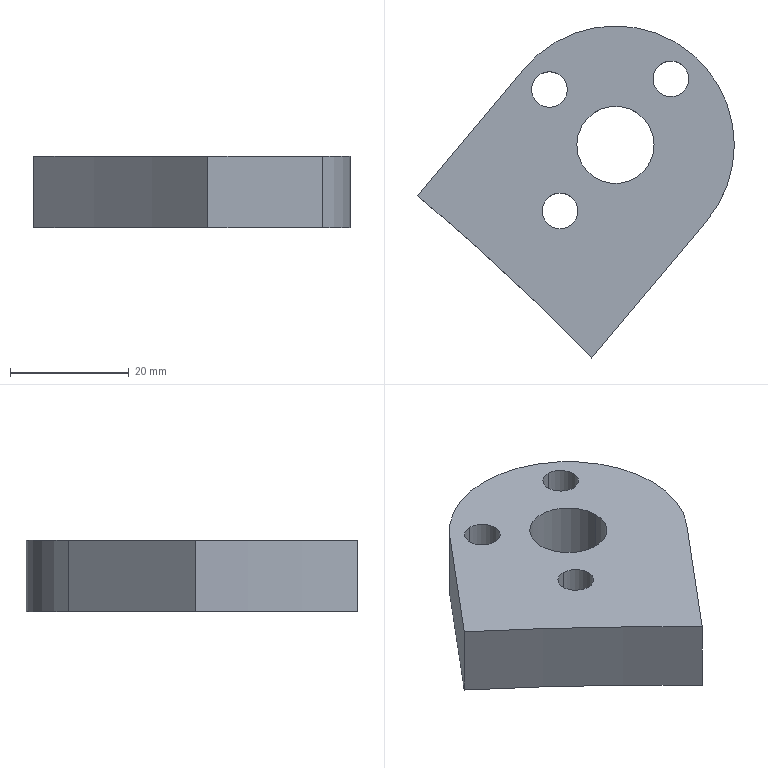Part | SolidWorks | features Extrusion 1, ICE 1 | 1 solid | 14 faces | box 53.274 x 55.837 x 12 mm | volume 18666 mm3 | cylinder 10 | plane 4 | commonest cylinder face diameters 6 x6 13 x2 40 x1 775 x1
STEP:
#1=CARTESIAN_POINT('',(291.675,319.49,6.));
#2=VERTEX_POINT('',#1);
#3=CARTESIAN_POINT('',(291.675,313.49,6.));
#4=VERTEX_POINT('',#3);
#5=CARTESIAN_POINT('',(291.675,316.49,6.));
#6=DIRECTION('',(0.,0.,1.));
#7=DIRECTION('',(-1.,0.,0.));
#8=AXIS2_PLACEMENT_3D('',#5,#6,#7);
#9=CIRCLE('',#8,3.);
#10=EDGE_CURVE('',#2,#4,#9,.T.);
#11=ORIENTED_EDGE('',*,*,#10,.T.);
#12=CARTESIAN_POINT('',(291.675,313.49,-6.));
#13=VERTEX_POINT('',#12);
#14=CARTESIAN_POINT('',(291.675,313.49,14.485));
#15=DIRECTION('',(0.,0.,-1.));
#16=VECTOR('',#15,1000.);
#17=LINE('',#14,#16);
#18=EDGE_CURVE('',#4,#13,#17,.T.);
#19=ORIENTED_EDGE('',*,*,#18,.T.);
#20=CARTESIAN_POINT('',(291.675,319.49,-6.));
#21=VERTEX_POINT('',#20);
#22=CARTESIAN_POINT('',(291.675,316.49,-6.));
#23=DIRECTION('',(0.,0.,-1.));
#24=DIRECTION('',(0.,1.,0.));
#25=AXIS2_PLACEMENT_3D('',#22,#23,#24);
#26=CIRCLE('',#25,3.);
#27=EDGE_CURVE('',#13,#21,#26,.T.);
#28=ORIENTED_EDGE('',*,*,#27,.T.);
#29=CARTESIAN_POINT('',(291.675,319.49,14.485));
#30=DIRECTION('',(0.,0.,-1.));
#31=VECTOR('',#30,1000.);
#32=LINE('',#29,#31);
#33=EDGE_CURVE('',#2,#21,#32,.T.);
#34=ORIENTED_EDGE('',*,*,#33,.F.);
#35=EDGE_LOOP('',(#11,#19,#28,#34));
#36=FACE_OUTER_BOUND('',#35,.T.);
#37=CARTESIAN_POINT('',(291.675,316.49,14.485));
#38=DIRECTION('',(0.,0.,-1.));
#39=DIRECTION('',(0.,1.,0.));
#40=AXIS2_PLACEMENT_3D('',#37,#38,#39);
#41=CYLINDRICAL_SURFACE('',#40,3.);
#42=ADVANCED_FACE('',(#36),#41,.F.);
#43=CARTESIAN_POINT('',(271.246,317.702,6.));
#44=VERTEX_POINT('',#43);
#45=CARTESIAN_POINT('',(271.246,311.702,6.));
#46=VERTEX_POINT('',#45);
#47=CARTESIAN_POINT('',(271.246,314.702,6.));
#48=DIRECTION('',(0.,0.,1.));
#49=DIRECTION('',(-1.,0.,0.));
#50=AXIS2_PLACEMENT_3D('',#47,#48,#49);
#51=CIRCLE('',#50,3.);
#52=EDGE_CURVE('',#44,#46,#51,.T.);
#53=ORIENTED_EDGE('',*,*,#52,.T.);
#54=CARTESIAN_POINT('',(271.246,311.702,-6.));
#55=VERTEX_POINT('',#54);
#56=CARTESIAN_POINT('',(271.246,311.702,14.485));
#57=DIRECTION('',(0.,0.,-1.));
#58=VECTOR('',#57,1000.);
#59=LINE('',#56,#58);
#60=EDGE_CURVE('',#46,#55,#59,.T.);
#61=ORIENTED_EDGE('',*,*,#60,.T.);
#62=CARTESIAN_POINT('',(271.246,317.702,-6.));
#63=VERTEX_POINT('',#62);
#64=CARTESIAN_POINT('',(271.246,314.702,-6.));
#65=DIRECTION('',(0.,0.,-1.));
#66=DIRECTION('',(0.,1.,0.));
#67=AXIS2_PLACEMENT_3D('',#64,#65,#66);
#68=CIRCLE('',#67,3.);
#69=EDGE_CURVE('',#55,#63,#68,.T.);
#70=ORIENTED_EDGE('',*,*,#69,.T.);
#71=CARTESIAN_POINT('',(271.246,317.702,14.485));
#72=DIRECTION('',(0.,0.,-1.));
#73=VECTOR('',#72,1000.);
#74=LINE('',#71,#73);
#75=EDGE_CURVE('',#44,#63,#74,.T.);
#76=ORIENTED_EDGE('',*,*,#75,.F.);
#77=EDGE_LOOP('',(#53,#61,#70,#76));
#78=FACE_OUTER_BOUND('',#77,.T.);
#79=CARTESIAN_POINT('',(271.246,314.702,14.485));
#80=DIRECTION('',(0.,0.,-1.));
#81=DIRECTION('',(0.,1.,0.));
#82=AXIS2_PLACEMENT_3D('',#79,#80,#81);
#83=CYLINDRICAL_SURFACE('',#82,3.);
#84=ADVANCED_FACE('',(#78),#83,.F.);
#85=CARTESIAN_POINT('',(273.034,297.274,6.));
#86=VERTEX_POINT('',#85);
#87=CARTESIAN_POINT('',(273.034,291.274,6.));
#88=VERTEX_POINT('',#87);
#89=CARTESIAN_POINT('',(273.034,294.274,6.));
#90=DIRECTION('',(0.,0.,1.));
#91=DIRECTION('',(-1.,0.,0.));
#92=AXIS2_PLACEMENT_3D('',#89,#90,#91);
#93=CIRCLE('',#92,3.);
#94=EDGE_CURVE('',#86,#88,#93,.T.);
#95=ORIENTED_EDGE('',*,*,#94,.T.);
#96=CARTESIAN_POINT('',(273.034,291.274,-6.));
#97=VERTEX_POINT('',#96);
#98=CARTESIAN_POINT('',(273.034,291.274,14.485));
#99=DIRECTION('',(0.,0.,-1.));
#100=VECTOR('',#99,1000.);
#101=LINE('',#98,#100);
#102=EDGE_CURVE('',#88,#97,#101,.T.);
#103=ORIENTED_EDGE('',*,*,#102,.T.);
#104=CARTESIAN_POINT('',(273.034,297.274,-6.));
#105=VERTEX_POINT('',#104);
#106=CARTESIAN_POINT('',(273.034,294.274,-6.));
#107=DIRECTION('',(0.,0.,-1.));
#108=DIRECTION('',(0.,1.,0.));
#109=AXIS2_PLACEMENT_3D('',#106,#107,#108);
#110=CIRCLE('',#109,3.);
#111=EDGE_CURVE('',#97,#105,#110,.T.);
#112=ORIENTED_EDGE('',*,*,#111,.T.);
#113=CARTESIAN_POINT('',(273.034,297.274,14.485));
#114=DIRECTION('',(0.,0.,-1.));
#115=VECTOR('',#114,1000.);
#116=LINE('',#113,#115);
#117=EDGE_CURVE('',#86,#105,#116,.T.);
#118=ORIENTED_EDGE('',*,*,#117,.F.);
#119=EDGE_LOOP('',(#95,#103,#112,#118));
#120=FACE_OUTER_BOUND('',#119,.T.);
#121=CARTESIAN_POINT('',(273.034,294.274,14.485));
#122=DIRECTION('',(0.,0.,-1.));
#123=DIRECTION('',(0.,1.,0.));
#124=AXIS2_PLACEMENT_3D('',#121,#122,#123);
#125=CYLINDRICAL_SURFACE('',#124,3.);
#126=ADVANCED_FACE('',(#120),#125,.F.);
#127=CARTESIAN_POINT('',(275.854,305.382,6.));
#128=VERTEX_POINT('',#127);
#129=CARTESIAN_POINT('',(288.854,305.382,6.));
#130=VERTEX_POINT('',#129);
#131=CARTESIAN_POINT('',(282.354,305.382,6.));
#132=DIRECTION('',(0.,0.,1.));
#133=DIRECTION('',(1.,0.,0.));
#134=AXIS2_PLACEMENT_3D('',#131,#132,#133);
#135=CIRCLE('',#134,6.5);
#136=EDGE_CURVE('',#128,#130,#135,.T.);
#137=ORIENTED_EDGE('',*,*,#136,.T.);
#138=CARTESIAN_POINT('',(288.854,305.382,-6.));
#139=VERTEX_POINT('',#138);
#140=CARTESIAN_POINT('',(288.854,305.382,6.));
#141=DIRECTION('',(0.,0.,-1.));
#142=VECTOR('',#141,1000.);
#143=LINE('',#140,#142);
#144=EDGE_CURVE('',#130,#139,#143,.T.);
#145=ORIENTED_EDGE('',*,*,#144,.T.);
#146=CARTESIAN_POINT('',(275.854,305.382,-6.));
#147=VERTEX_POINT('',#146);
#148=CARTESIAN_POINT('',(282.354,305.382,-6.));
#149=DIRECTION('',(0.,0.,1.));
#150=DIRECTION('',(1.,0.,0.));
#151=AXIS2_PLACEMENT_3D('',#148,#149,#150);
#152=CIRCLE('',#151,6.5);
#153=EDGE_CURVE('',#147,#139,#152,.T.);
#154=ORIENTED_EDGE('',*,*,#153,.F.);
#155=CARTESIAN_POINT('',(275.854,305.382,6.));
#156=DIRECTION('',(0.,0.,-1.));
#157=VECTOR('',#156,1000.);
#158=LINE('',#155,#157);
#159=EDGE_CURVE('',#128,#147,#158,.T.);
#160=ORIENTED_EDGE('',*,*,#159,.F.);
#161=EDGE_LOOP('',(#137,#145,#154,#160));
#162=FACE_OUTER_BOUND('',#161,.T.);
#163=CARTESIAN_POINT('',(282.354,305.382,6.));
#164=DIRECTION('',(0.,0.,-1.));
#165=DIRECTION('',(-1.,0.,0.));
#166=AXIS2_PLACEMENT_3D('',#163,#164,#165);
#167=CYLINDRICAL_SURFACE('',#166,6.5);
#168=ADVANCED_FACE('',(#162),#167,.F.);
#169=ORIENTED_EDGE('',*,*,#10,.F.);
#170=CARTESIAN_POINT('',(291.675,316.49,6.));
#171=DIRECTION('',(0.,0.,1.));
#172=DIRECTION('',(-1.,0.,0.));
#173=AXIS2_PLACEMENT_3D('',#170,#171,#172);
#174=CIRCLE('',#173,3.);
#175=EDGE_CURVE('',#4,#2,#174,.T.);
#176=ORIENTED_EDGE('',*,*,#175,.F.);
#177=EDGE_LOOP('',(#169,#176));
#178=FACE_BOUND('',#177,.T.);
#179=ORIENTED_EDGE('',*,*,#52,.F.);
#180=CARTESIAN_POINT('',(271.246,314.702,6.));
#181=DIRECTION('',(0.,0.,1.));
#182=DIRECTION('',(-1.,0.,0.));
#183=AXIS2_PLACEMENT_3D('',#180,#181,#182);
#184=CIRCLE('',#183,3.);
#185=EDGE_CURVE('',#46,#44,#184,.T.);
#186=ORIENTED_EDGE('',*,*,#185,.F.);
#187=EDGE_LOOP('',(#179,#186));
#188=FACE_BOUND('',#187,.T.);
#189=ORIENTED_EDGE('',*,*,#94,.F.);
#190=CARTESIAN_POINT('',(273.034,294.274,6.));
#191=DIRECTION('',(0.,0.,1.));
#192=DIRECTION('',(-1.,0.,0.));
#193=AXIS2_PLACEMENT_3D('',#190,#191,#192);
#194=CIRCLE('',#193,3.);
#195=EDGE_CURVE('',#88,#86,#194,.T.);
#196=ORIENTED_EDGE('',*,*,#195,.F.);
#197=EDGE_LOOP('',(#189,#196));
#198=FACE_BOUND('',#197,.T.);
#199=CARTESIAN_POINT('',(249.08,296.842,6.));
#200=VERTEX_POINT('',#199);
#201=CARTESIAN_POINT('',(278.391,269.545,6.));
#202=VERTEX_POINT('',#201);
#203=CARTESIAN_POINT('',(0.,0.,6.));
#204=DIRECTION('',(0.,0.,-1.));
#205=DIRECTION('',(-1.,0.,0.));
#206=AXIS2_PLACEMENT_3D('',#203,#204,#205);
#207=CIRCLE('',#206,387.5);
#208=EDGE_CURVE('',#200,#202,#207,.T.);
#209=ORIENTED_EDGE('',*,*,#208,.T.);
#210=CARTESIAN_POINT('',(297.675,292.526,6.));
#211=VERTEX_POINT('',#210);
#212=CARTESIAN_POINT('',(278.391,269.545,6.));
#213=DIRECTION('',(0.6428,0.766,0.));
#214=VECTOR('',#213,1000.);
#215=LINE('',#212,#214);
#216=EDGE_CURVE('',#202,#211,#215,.T.);
#217=ORIENTED_EDGE('',*,*,#216,.T.);
#218=CARTESIAN_POINT('',(267.033,318.238,6.));
#219=VERTEX_POINT('',#218);
#220=CARTESIAN_POINT('',(282.354,305.382,6.));
#221=DIRECTION('',(0.,0.,1.));
#222=DIRECTION('',(-1.,0.,0.));
#223=AXIS2_PLACEMENT_3D('',#220,#221,#222);
#224=CIRCLE('',#223,20.);
#225=EDGE_CURVE('',#211,#219,#224,.T.);
#226=ORIENTED_EDGE('',*,*,#225,.T.);
#227=CARTESIAN_POINT('',(249.08,296.842,6.));
#228=DIRECTION('',(-0.6428,-0.766,0.));
#229=VECTOR('',#228,1000.);
#230=LINE('',#227,#229);
#231=EDGE_CURVE('',#219,#200,#230,.T.);
#232=ORIENTED_EDGE('',*,*,#231,.T.);
#233=EDGE_LOOP('',(#209,#217,#226,#232));
#234=FACE_OUTER_BOUND('',#233,.T.);
#235=ORIENTED_EDGE('',*,*,#136,.F.);
#236=CARTESIAN_POINT('',(282.354,305.382,6.));
#237=DIRECTION('',(0.,0.,1.));
#238=DIRECTION('',(1.,0.,0.));
#239=AXIS2_PLACEMENT_3D('',#236,#237,#238);
#240=CIRCLE('',#239,6.5);
#241=EDGE_CURVE('',#130,#128,#240,.T.);
#242=ORIENTED_EDGE('',*,*,#241,.F.);
#243=EDGE_LOOP('',(#235,#242));
#244=FACE_BOUND('',#243,.T.);
#245=CARTESIAN_POINT('',(0.,0.,6.));
#246=DIRECTION('',(0.,0.,-1.));
#247=DIRECTION('',(-1.,0.,0.));
#248=AXIS2_PLACEMENT_3D('',#245,#246,#247);
#249=PLANE('',#248);
#250=ADVANCED_FACE('',(#178,#188,#198,#234,#244),#249,.F.);
#251=CARTESIAN_POINT('',(291.675,316.49,-6.));
#252=DIRECTION('',(0.,0.,-1.));
#253=DIRECTION('',(0.,1.,0.));
#254=AXIS2_PLACEMENT_3D('',#251,#252,#253);
#255=CIRCLE('',#254,3.);
#256=EDGE_CURVE('',#21,#13,#255,.T.);
#257=ORIENTED_EDGE('',*,*,#256,.F.);
#258=ORIENTED_EDGE('',*,*,#27,.F.);
#259=EDGE_LOOP('',(#257,#258));
#260=FACE_BOUND('',#259,.T.);
#261=CARTESIAN_POINT('',(271.246,314.702,-6.));
#262=DIRECTION('',(0.,0.,-1.));
#263=DIRECTION('',(0.,1.,0.));
#264=AXIS2_PLACEMENT_3D('',#261,#262,#263);
#265=CIRCLE('',#264,3.);
#266=EDGE_CURVE('',#63,#55,#265,.T.);
#267=ORIENTED_EDGE('',*,*,#266,.F.);
#268=ORIENTED_EDGE('',*,*,#69,.F.);
#269=EDGE_LOOP('',(#267,#268));
#270=FACE_BOUND('',#269,.T.);
#271=CARTESIAN_POINT('',(273.034,294.274,-6.));
#272=DIRECTION('',(0.,0.,-1.));
#273=DIRECTION('',(0.,1.,0.));
#274=AXIS2_PLACEMENT_3D('',#271,#272,#273);
#275=CIRCLE('',#274,3.);
#276=EDGE_CURVE('',#105,#97,#275,.T.);
#277=ORIENTED_EDGE('',*,*,#276,.F.);
#278=ORIENTED_EDGE('',*,*,#111,.F.);
#279=EDGE_LOOP('',(#277,#278));
#280=FACE_BOUND('',#279,.T.);
#281=CARTESIAN_POINT('',(249.08,296.842,-6.));
#282=VERTEX_POINT('',#281);
#283=CARTESIAN_POINT('',(278.391,269.545,-6.));
#284=VERTEX_POINT('',#283);
#285=CARTESIAN_POINT('',(0.,0.,-6.));
#286=DIRECTION('',(0.,0.,-1.));
#287=DIRECTION('',(-1.,0.,0.));
#288=AXIS2_PLACEMENT_3D('',#285,#286,#287);
#289=CIRCLE('',#288,387.5);
#290=EDGE_CURVE('',#282,#284,#289,.T.);
#291=ORIENTED_EDGE('',*,*,#290,.F.);
#292=CARTESIAN_POINT('',(267.033,318.238,-6.));
#293=VERTEX_POINT('',#292);
#294=CARTESIAN_POINT('',(249.08,296.842,-6.));
#295=DIRECTION('',(-0.6428,-0.766,0.));
#296=VECTOR('',#295,1000.);
#297=LINE('',#294,#296);
#298=EDGE_CURVE('',#293,#282,#297,.T.);
#299=ORIENTED_EDGE('',*,*,#298,.F.);
#300=CARTESIAN_POINT('',(297.675,292.526,-6.));
#301=VERTEX_POINT('',#300);
#302=CARTESIAN_POINT('',(282.354,305.382,-6.));
#303=DIRECTION('',(0.,0.,1.));
#304=DIRECTION('',(-1.,0.,0.));
#305=AXIS2_PLACEMENT_3D('',#302,#303,#304);
#306=CIRCLE('',#305,20.);
#307=EDGE_CURVE('',#301,#293,#306,.T.);
#308=ORIENTED_EDGE('',*,*,#307,.F.);
#309=CARTESIAN_POINT('',(278.391,269.545,-6.));
#310=DIRECTION('',(0.6428,0.766,0.));
#311=VECTOR('',#310,1000.);
#312=LINE('',#309,#311);
#313=EDGE_CURVE('',#284,#301,#312,.T.);
#314=ORIENTED_EDGE('',*,*,#313,.F.);
#315=EDGE_LOOP('',(#291,#299,#308,#314));
#316=FACE_OUTER_BOUND('',#315,.T.);
#317=ORIENTED_EDGE('',*,*,#153,.T.);
#318=CARTESIAN_POINT('',(282.354,305.382,-6.));
#319=DIRECTION('',(0.,0.,1.));
#320=DIRECTION('',(1.,0.,0.));
#321=AXIS2_PLACEMENT_3D('',#318,#319,#320);
#322=CIRCLE('',#321,6.5);
#323=EDGE_CURVE('',#139,#147,#322,.T.);
#324=ORIENTED_EDGE('',*,*,#323,.T.);
#325=EDGE_LOOP('',(#317,#324));
#326=FACE_BOUND('',#325,.T.);
#327=CARTESIAN_POINT('',(0.,0.,-6.));
#328=DIRECTION('',(0.,0.,-1.));
#329=DIRECTION('',(-1.,0.,0.));
#330=AXIS2_PLACEMENT_3D('',#327,#328,#329);
#331=PLANE('',#330);
#332=ADVANCED_FACE('',(#260,#270,#280,#316,#326),#331,.T.);
#333=ORIENTED_EDGE('',*,*,#290,.T.);
#334=CARTESIAN_POINT('',(278.391,269.545,6.));
#335=DIRECTION('',(0.,0.,-1.));
#336=VECTOR('',#335,1000.);
#337=LINE('',#334,#336);
#338=EDGE_CURVE('',#202,#284,#337,.T.);
#339=ORIENTED_EDGE('',*,*,#338,.F.);
#340=ORIENTED_EDGE('',*,*,#208,.F.);
#341=CARTESIAN_POINT('',(249.08,296.842,6.));
#342=DIRECTION('',(0.,0.,-1.));
#343=VECTOR('',#342,1000.);
#344=LINE('',#341,#343);
#345=EDGE_CURVE('',#200,#282,#344,.T.);
#346=ORIENTED_EDGE('',*,*,#345,.T.);
#347=EDGE_LOOP('',(#333,#339,#340,#346));
#348=FACE_OUTER_BOUND('',#347,.T.);
#349=CARTESIAN_POINT('',(0.,0.,6.));
#350=DIRECTION('',(0.,0.,-1.));
#351=DIRECTION('',(-1.,0.,0.));
#352=AXIS2_PLACEMENT_3D('',#349,#350,#351);
#353=CYLINDRICAL_SURFACE('',#352,387.5);
#354=ADVANCED_FACE('',(#348),#353,.F.);
#355=ORIENTED_EDGE('',*,*,#313,.T.);
#356=CARTESIAN_POINT('',(297.675,292.526,6.));
#357=DIRECTION('',(0.,0.,-1.));
#358=VECTOR('',#357,1000.);
#359=LINE('',#356,#358);
#360=EDGE_CURVE('',#211,#301,#359,.T.);
#361=ORIENTED_EDGE('',*,*,#360,.F.);
#362=ORIENTED_EDGE('',*,*,#216,.F.);
#363=ORIENTED_EDGE('',*,*,#338,.T.);
#364=EDGE_LOOP('',(#355,#361,#362,#363));
#365=FACE_OUTER_BOUND('',#364,.T.);
#366=CARTESIAN_POINT('',(278.391,269.545,6.));
#367=DIRECTION('',(-0.766,0.6428,0.));
#368=DIRECTION('',(-0.6428,-0.766,0.));
#369=AXIS2_PLACEMENT_3D('',#366,#367,#368);
#370=PLANE('',#369);
#371=ADVANCED_FACE('',(#365),#370,.F.);
#372=ORIENTED_EDGE('',*,*,#307,.T.);
#373=CARTESIAN_POINT('',(267.033,318.238,6.));
#374=DIRECTION('',(0.,0.,-1.));
#375=VECTOR('',#374,1000.);
#376=LINE('',#373,#375);
#377=EDGE_CURVE('',#219,#293,#376,.T.);
#378=ORIENTED_EDGE('',*,*,#377,.F.);
#379=ORIENTED_EDGE('',*,*,#225,.F.);
#380=ORIENTED_EDGE('',*,*,#360,.T.);
#381=EDGE_LOOP('',(#372,#378,#379,#380));
#382=FACE_OUTER_BOUND('',#381,.T.);
#383=CARTESIAN_POINT('',(282.354,305.382,6.));
#384=DIRECTION('',(0.,0.,-1.));
#385=DIRECTION('',(-1.,0.,0.));
#386=AXIS2_PLACEMENT_3D('',#383,#384,#385);
#387=CYLINDRICAL_SURFACE('',#386,20.);
#388=ADVANCED_FACE('',(#382),#387,.T.);
#389=ORIENTED_EDGE('',*,*,#298,.T.);
#390=ORIENTED_EDGE('',*,*,#345,.F.);
#391=ORIENTED_EDGE('',*,*,#231,.F.);
#392=ORIENTED_EDGE('',*,*,#377,.T.);
#393=EDGE_LOOP('',(#389,#390,#391,#392));
#394=FACE_OUTER_BOUND('',#393,.T.);
#395=CARTESIAN_POINT('',(249.08,296.842,6.));
#396=DIRECTION('',(0.766,-0.6428,0.));
#397=DIRECTION('',(0.6428,0.766,0.));
#398=AXIS2_PLACEMENT_3D('',#395,#396,#397);
#399=PLANE('',#398);
#400=ADVANCED_FACE('',(#394),#399,.F.);
#401=ORIENTED_EDGE('',*,*,#144,.F.);
#402=ORIENTED_EDGE('',*,*,#241,.T.);
#403=ORIENTED_EDGE('',*,*,#159,.T.);
#404=ORIENTED_EDGE('',*,*,#323,.F.);
#405=EDGE_LOOP('',(#401,#402,#403,#404));
#406=FACE_OUTER_BOUND('',#405,.T.);
#407=CARTESIAN_POINT('',(282.354,305.382,6.));
#408=DIRECTION('',(0.,0.,-1.));
#409=DIRECTION('',(-1.,0.,0.));
#410=AXIS2_PLACEMENT_3D('',#407,#408,#409);
#411=CYLINDRICAL_SURFACE('',#410,6.5);
#412=ADVANCED_FACE('',(#406),#411,.F.);
#413=ORIENTED_EDGE('',*,*,#102,.F.);
#414=ORIENTED_EDGE('',*,*,#195,.T.);
#415=ORIENTED_EDGE('',*,*,#117,.T.);
#416=ORIENTED_EDGE('',*,*,#276,.T.);
#417=EDGE_LOOP('',(#413,#414,#415,#416));
#418=FACE_OUTER_BOUND('',#417,.T.);
#419=CARTESIAN_POINT('',(273.034,294.274,14.485));
#420=DIRECTION('',(0.,0.,-1.));
#421=DIRECTION('',(0.,1.,0.));
#422=AXIS2_PLACEMENT_3D('',#419,#420,#421);
#423=CYLINDRICAL_SURFACE('',#422,3.);
#424=ADVANCED_FACE('',(#418),#423,.F.);
#425=ORIENTED_EDGE('',*,*,#60,.F.);
#426=ORIENTED_EDGE('',*,*,#185,.T.);
#427=ORIENTED_EDGE('',*,*,#75,.T.);
#428=ORIENTED_EDGE('',*,*,#266,.T.);
#429=EDGE_LOOP('',(#425,#426,#427,#428));
#430=FACE_OUTER_BOUND('',#429,.T.);
#431=CARTESIAN_POINT('',(271.246,314.702,14.485));
#432=DIRECTION('',(0.,0.,-1.));
#433=DIRECTION('',(0.,1.,0.));
#434=AXIS2_PLACEMENT_3D('',#431,#432,#433);
#435=CYLINDRICAL_SURFACE('',#434,3.);
#436=ADVANCED_FACE('',(#430),#435,.F.);
#437=ORIENTED_EDGE('',*,*,#18,.F.);
#438=ORIENTED_EDGE('',*,*,#175,.T.);
#439=ORIENTED_EDGE('',*,*,#33,.T.);
#440=ORIENTED_EDGE('',*,*,#256,.T.);
#441=EDGE_LOOP('',(#437,#438,#439,#440));
#442=FACE_OUTER_BOUND('',#441,.T.);
#443=CARTESIAN_POINT('',(291.675,316.49,14.485));
#444=DIRECTION('',(0.,0.,-1.));
#445=DIRECTION('',(0.,1.,0.));
#446=AXIS2_PLACEMENT_3D('',#443,#444,#445);
#447=CYLINDRICAL_SURFACE('',#446,3.);
#448=ADVANCED_FACE('',(#442),#447,.F.);
#449=CLOSED_SHELL('',(#42,#84,#126,#168,#250,#332,#354,#371,#388,#400,#412,#424,#436,#448));
#450=MANIFOLD_SOLID_BREP('',#449);
#451=CARTESIAN_POINT('',(0.,0.,0.));
#452=DIRECTION('',(0.,0.,1.));
#453=DIRECTION('',(1.,0.,0.));
#454=AXIS2_PLACEMENT_3D('',#451,#452,#453);
#455=(LENGTH_UNIT()NAMED_UNIT(*)SI_UNIT(.MILLI.,.METRE.));
#456=UNCERTAINTY_MEASURE_WITH_UNIT(LENGTH_MEASURE(0.00001),#455,'','');
#457=(NAMED_UNIT(*)PLANE_ANGLE_UNIT()SI_UNIT($,.RADIAN.));
#458=(NAMED_UNIT(*)SI_UNIT($,.STERADIAN.)SOLID_ANGLE_UNIT());
#459=(GEOMETRIC_REPRESENTATION_CONTEXT(3)GLOBAL_UNCERTAINTY_ASSIGNED_CONTEXT((#456))GLOBAL_UNIT_ASSIGNED_CONTEXT((#455,#457,#458))REPRESENTATION_CONTEXT('',''));
#460=ADVANCED_BREP_SHAPE_REPRESENTATION('',(#450,#454),#459);